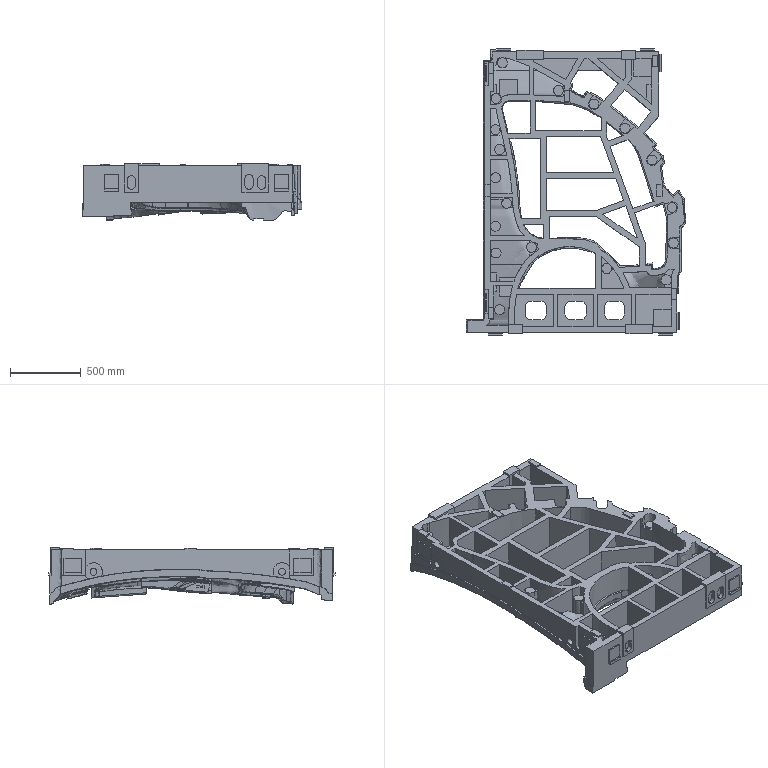Part | NX | features solid 2 | 1 solid | 2093 faces | box 1547 x 2020 x 402.676 mm | volume 283620447 mm3 | spline 1131 | plane 539 | cylinder 403 | torus 9 | sphere 7 | cone 4 | commonest cylinder face diameters 10 x63 6 x39 52 x24 80 x23 14 x20 20 x16